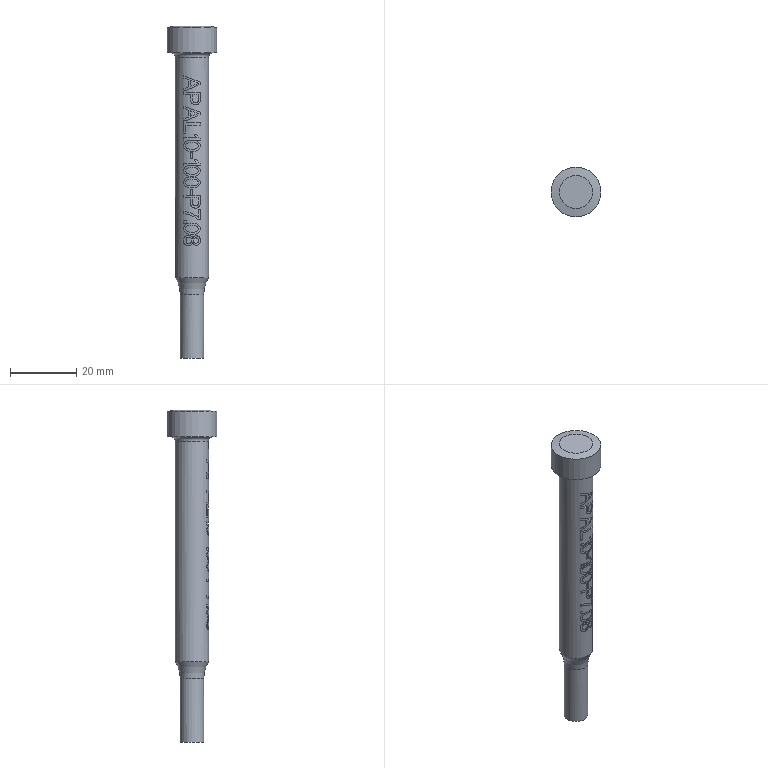Part | STEP file | PN_0052_id1718_x_t | 1 solid | 194 faces | box 15 x 15 x 100 mm | volume 7737 mm3 | plane 112 | cylinder 79 | torus 2 | cone 1 | commonest cylinder face diameters 9.8 x16 10 x11 2.089 x4 2.493 x4 2.5 x4 2.529 x4